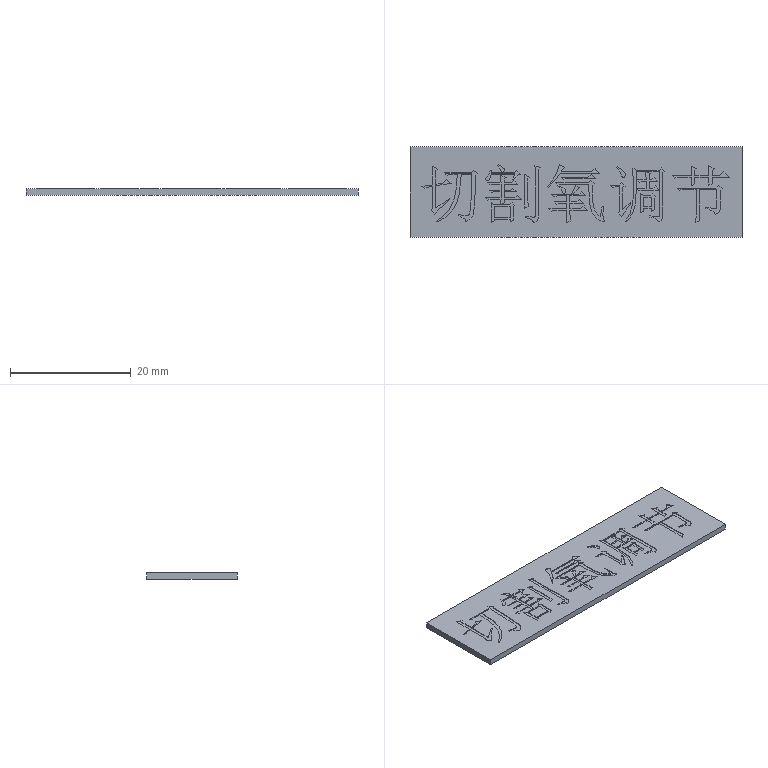Part | STEP file | HXGR200008-06-02-03 | 1 solid | 327 faces | box 55 x 15 x 1 mm | volume 815.181 mm3 | plane 249 | spline 78